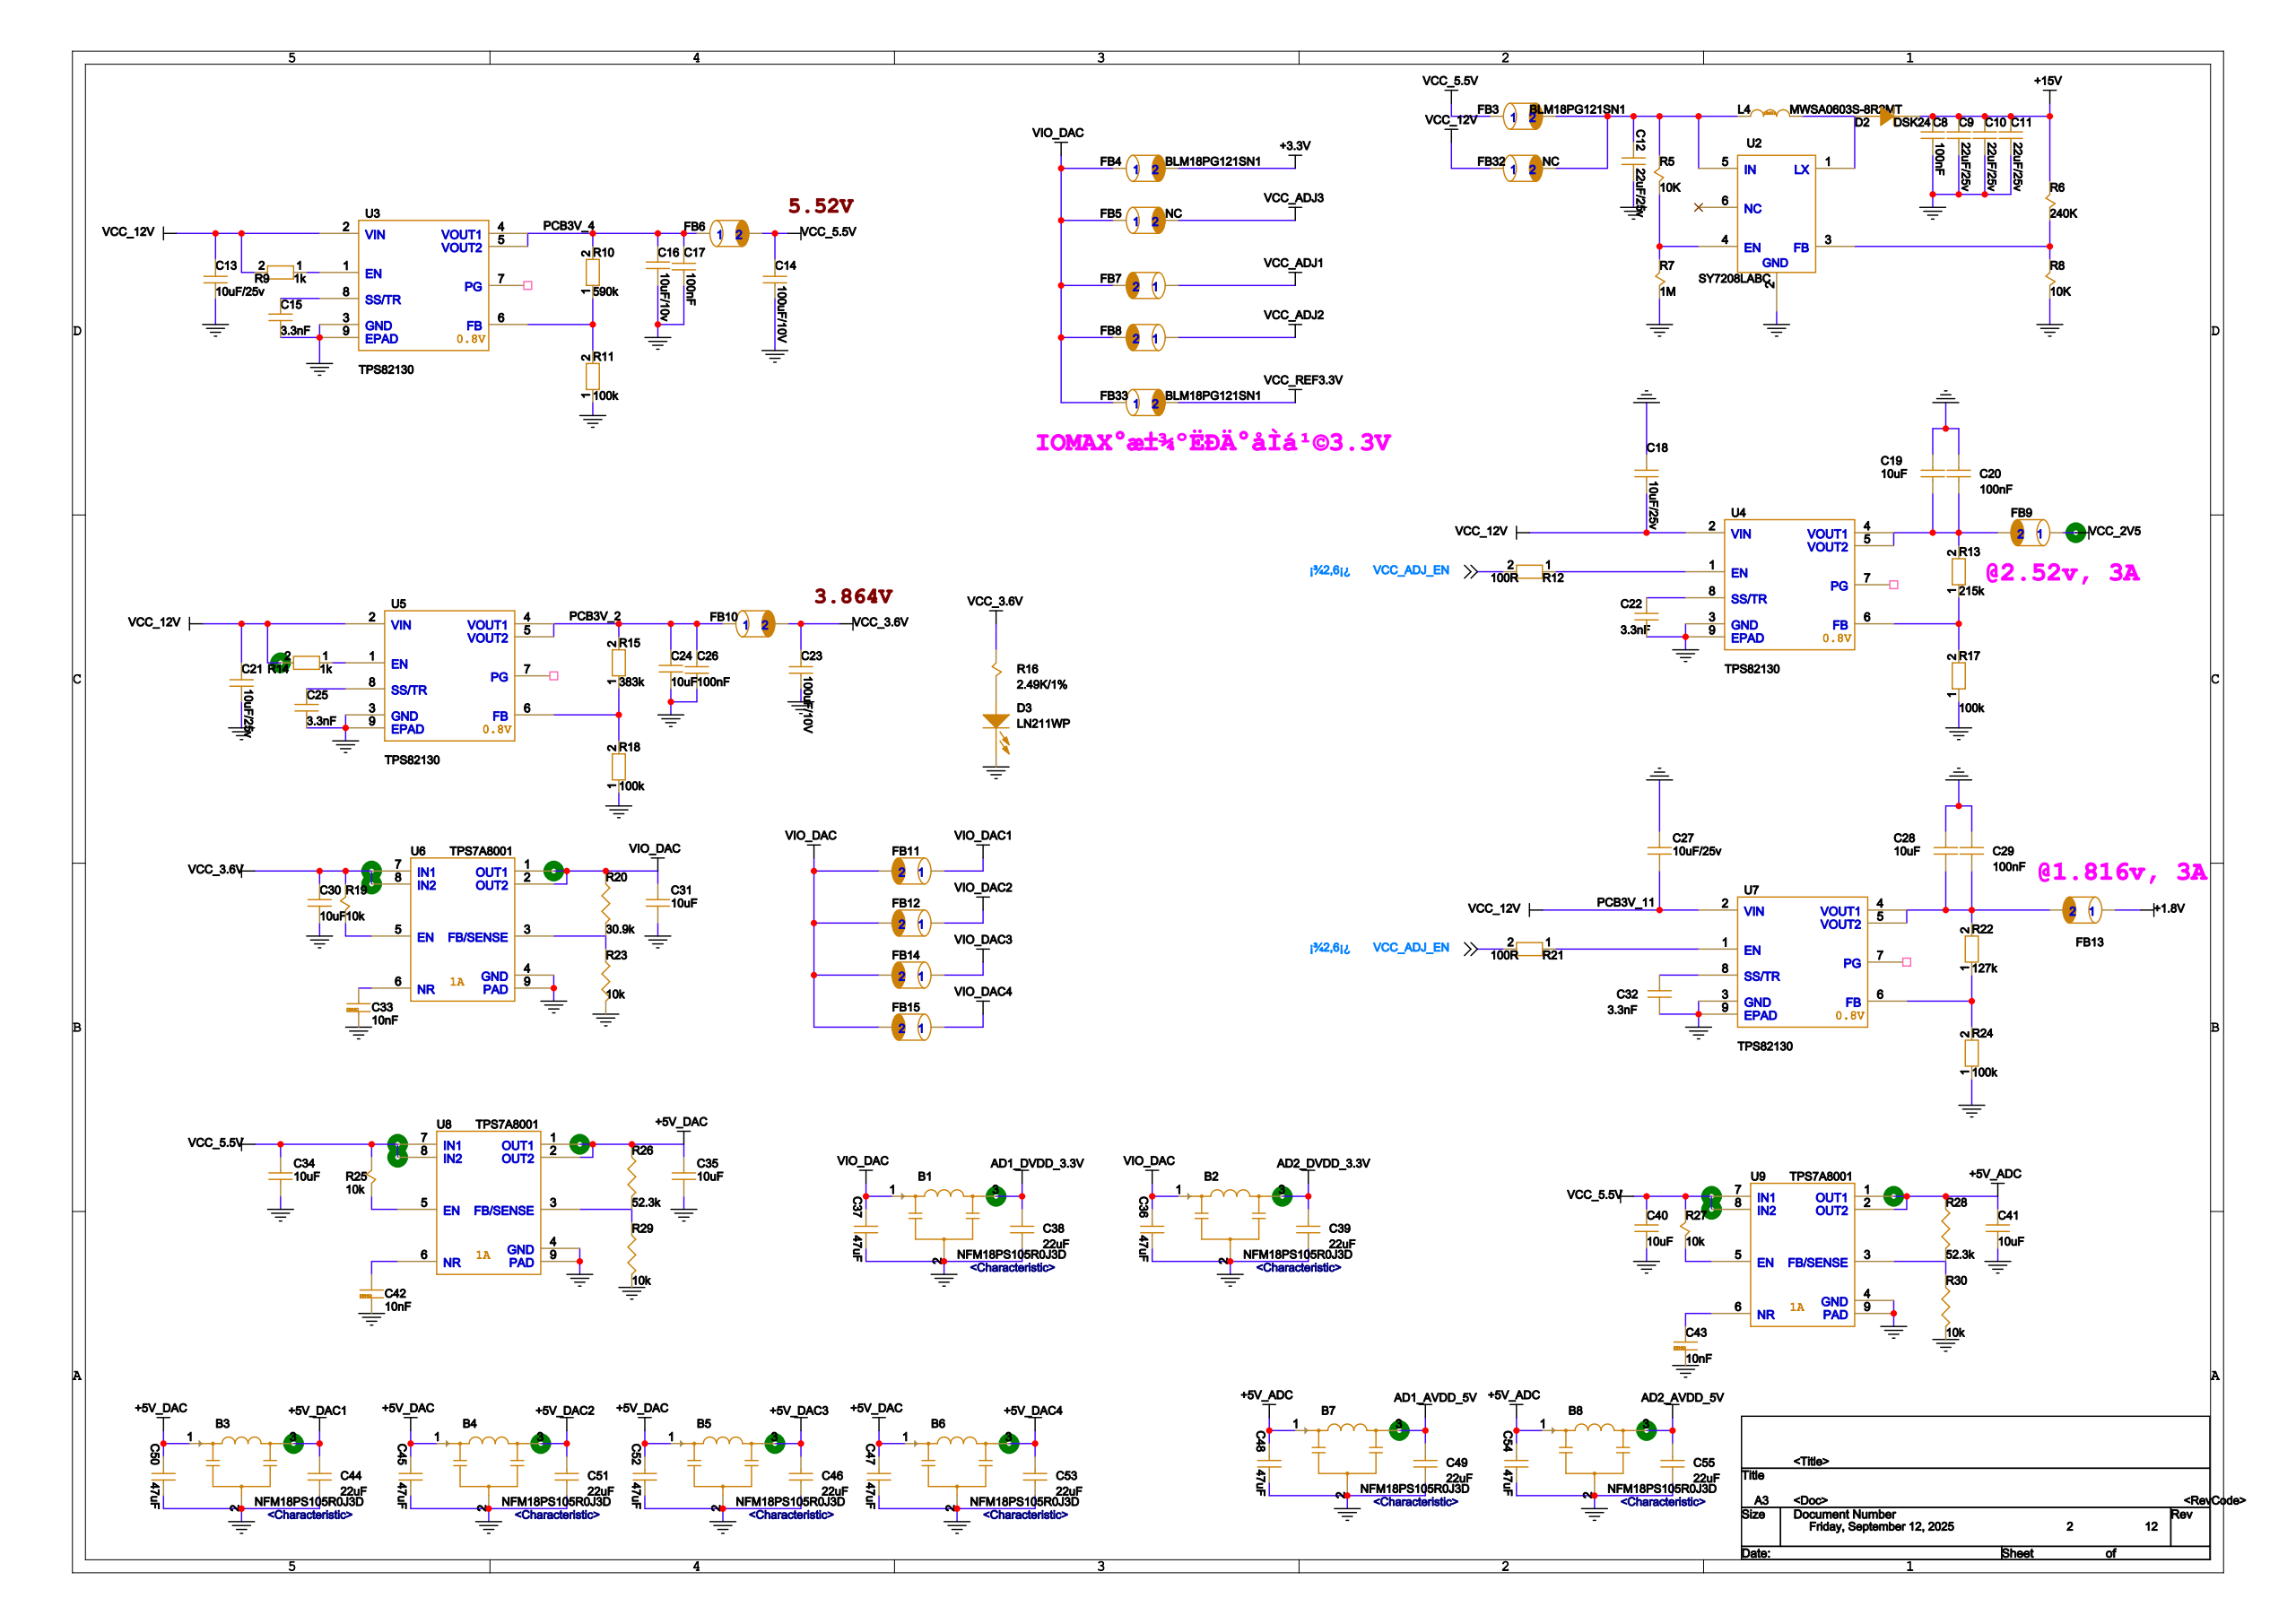Circuit board | Cadence Allegro | 528 parts | 530 nets | one sheet of the schematic
Parts on this sheet (reference | value | footprint):
B1 | NFM18PS105R0J3D | B0603
B2 | NFM18PS105R0J3D | B0603
B3 | NFM18PS105R0J3D | B0603
B4 | NFM18PS105R0J3D | B0603
B5 | NFM18PS105R0J3D | B0603
B6 | NFM18PS105R0J3D | B0603
B7 | NFM18PS105R0J3D | B0603
B8 | NFM18PS105R0J3D | B0603
C10 | 22uF/25v | C0805
C11 | 22uF/25v | C0805
C12 | 22uF/25v | C0805
C13 | 10uF/25v | C0805
C14 | 100uF/10V | C1210
C15 | 3.3nF | C0402
C16 | 10uF/10v | C0805
C17 | 100nF | C0402
C18 | 10uF/25v | C0805
C19 | 10uF | C0805
C20 | 100nF | C0402
C21 | 10uF/25v | C0805
C22 | 3.3nF | C0402
C23 | 100uF/10V | C1210
C24 | 10uF | C0805
C25 | 3.3nF | C0402
C26 | 100nF | C0402
C27 | 10uF/25v | C0805
C28 | 10uF | C0805
C29 | 100nF | C0402
C30 | 10uF | C0805
C31 | 10uF | C0805
C32 | 3.3nF | C0402
C33 | 10nF | C0402
C34 | 10uF | C0805
C35 | 10uF | C0805
C36 | 47uF | C0805
C37 | 47uF | C0805
C38 | 22uF | C0805
C39 | 22uF | C0805
C40 | 10uF | C0805
C41 | 10uF | C0805
C42 | 10nF | C0402
C43 | 10nF | C0402
C44 | 22uF | C0805
C45 | 47uF | C0805
C46 | 22uF | C0805
C47 | 47uF | C0805
C48 | 47uF | C0805
C49 | 22uF | C0805
C50 | 47uF | C0805
C51 | 22uF | C0805
C52 | 47uF | C0805
C53 | 22uF | C0805
C54 | 47uF | C0805
C55 | 22uF | C0805
D2 | DSK24 | DSK24
D3 | LN211WP | D0603
FB3 | BLM18PG121SN1 | 0603
FB4 | BLM18PG121SN1 | 0603
FB5 | NC | 0603
FB6 | BLM18PG121SN1 | 0603
FB7 | BLM18PG121SN1 | 0603
FB8 | BLM18PG121SN1 | 0603
FB9 | BLM18PG121SN1 | 0603
FB10 | BLM18PG121SN1 | 0603
FB11 | BLM18PG121SN1 | 0603
FB12 | BLM18PG121SN1 | 0603
FB13 | BLM18PG121SN1 | 0603
FB14 | BLM18PG121SN1 | 0603
FB15 | BLM18PG121SN1 | 0603
FB32 | NC | 0603
FB33 | BLM18PG121SN1 | 0603
L4 | MWSA0603S-8R2MT | PL0603
R5 | 10k | R0402
R6 | 240K | R0603
R7 | 1M | R0603
R8 | 10k | R0402
R9 | 1k | R0402
R10 | 590k | R0603
R11 | 100k | R0402
R12 | 100R | R0402
R13 | 215k | R0603
R14 | 1k | R0402
R15 | 383k | R0603
R16 | 2.49K/1% | R0402
R17 | 100k | R0402
R18 | 100k | R0402
R19 | 10k | R0402
R20 | 30.9k | R0402
R21 | 100R | R0402
R22 | 127k | R0603
R23 | 10k | R0402
R24 | 100k | R0402
R25 | 10k | R0402
R26 | 52.3k | R0402
R27 | 10k | R0402
R28 | 52.3k | R0402
R29 | 10k | R0402
R30 | 10k | R0402
U2 | SY7208LABC | SOT23-6
U3 | TPS82130 | SIL0008C
U4 | TPS82130 | SIL0008C
U5 | TPS82130 | SIL0008C
U6 | TPS7A8001 | TPS7A8001
U7 | TPS82130 | SIL0008C
U8 | TPS7A8001 | TPS7A8001
U9 | TPS7A8001 | TPS7A8001
Nets of these parts (net: part-pin ...):
N18761532: D2-2 L4-2 U2-1
+15V: C10-1 C11-1 D2-1 R6-1
GND: B1-2 B2-2 B3-2 B4-2 B5-2 B6-2 B7-2 B8-2 C10-2 C11-2 C12-2 C13-1 C14-1 C15-2 C16-2 C17-1 C18-1 C19-1 C20-1 C21-1 C22-2 C23-1 C24-2 C25-2 C26-1 C27-1 C28-1 C29-1 C30-2 C31-2 C32-2 C33-1 C34-2 C35-2 C36-1 C37-1 C38-1 C39-1 C40-2 C41-2 C42-1 C43-1 C44-1 C45-1 C46-1 C47-1 C48-1 C49-1 C50-1 C51-1 C52-1 C53-1 C54-1 C55-1 D3-2 R7-2 R8-2 R11-1 R17-1 R18-1 R23-2 R24-1 R29-2 R30-2 U2-2 U3-3 U3-9 U4-3 U4-9 U5-3 U5-9 U6-4 U6-9 U7-3 U7-9 U8-4 U8-9 U9-4 U9-9
AD1_AVDD_5V: B7-3 C49-2
AD1_DVDD_3.3V: B1-3 C38-2
AD2_AVDD_5V: B8-3 C55-2
AD2_DVDD_3.3V: B2-3 C39-2
VIO_DAC: B1-1 B2-1 C31-1 C36-2 C37-2 FB4-1 FB5-1 FB7-2 FB8-2 FB11-2 FB12-2 FB14-2 FB15-2 FB33-1 R20-1 U6-1 U6-2
+5V_DAC: B3-1 B4-1 B5-1 B6-1 C35-1 C45-2 C47-2 C50-2 C52-2 R26-1 U8-1 U8-2
+5V_DAC1: B3-3 C44-2
+5V_DAC2: B4-3 C51-2
+5V_DAC3: B5-3 C46-2
+5V_DAC4: B6-3 C53-2
+5V_ADC: B7-1 B8-1 C41-1 C48-2 C54-2 R28-1 U9-1 U9-2
VCC_REF3.3V: FB33-2
VCC_12V: C13-2 C18-2 C21-2 C27-2 FB32-1 R9-2 R14-2 U3-2 U4-2 U5-2 U7-2
N18757659: C12-1 FB3-2 FB32-2 L4-1 R5-2 U2-5
VCC_ADJ3: FB5-2
VCC_3.6V: C23-2 C30-1 FB10-2 R16-1 R19-2 U6-7 U6-8
N18730043: R19-1 U6-5
N18730051: R20-2 R23-1 U6-3
N18730069: C33-2 U6-6
N18728670: R25-1 U8-5
N18728678: R26-2 R29-1 U8-3
VCC_5.5V: C14-2 C34-1 C40-1 FB3-1 FB6-2 R25-2 R27-2 U8-7 U8-8 U9-7 U9-8
N18728694: C42-2 U8-6
N18732431: R27-1 U9-5
N18732439: R28-2 R30-1 U9-3
N18732455: C43-2 U9-6
+3.3V: FB4-2
PCB3V_4: C16-1 C17-2 FB6-1 R10-2 U3-4 U3-5
N18428547: C19-2 C20-2 FB9-2 R13-2 U4-4 U4-5
PCB3V_2: C24-1 C26-2 FB10-1 R15-2 U5-4 U5-5
N18528537: C28-2 C29-2 FB13-2 R22-2 U7-4 U7-5
VIO_DAC1: FB11-1
VIO_DAC2: FB12-1
VIO_DAC3: FB14-1
VIO_DAC4: FB15-1
N19806909: C15-1 U3-8
N18428651: C22-1 U4-8
N19932993: C25-1 U5-8
N19781738: C32-1 U7-8
N183130531: D3-1 R16-2
+1.8V: FB13-1
VCC_ADJ1: FB7-1
VCC_ADJ2: FB8-1
VCC_2V5: FB9-1
N19806911: R10-1 R11-2 U3-6
N18428653: R13-1 R17-2 U4-6
N19932995: R15-1 R18-2 U5-6
N19781740: R22-1 R24-2 U7-6
N18428657: R12-1 U4-1
VCC_ADJ_EN: R12-2 R21-2
N19781717: R21-1 U7-1
N19932991: R14-1 U5-1
N18731960: R9-1 U3-1
N18763447: R5-1 R7-1 U2-4
N18759407: R6-2 R8-1 U2-3